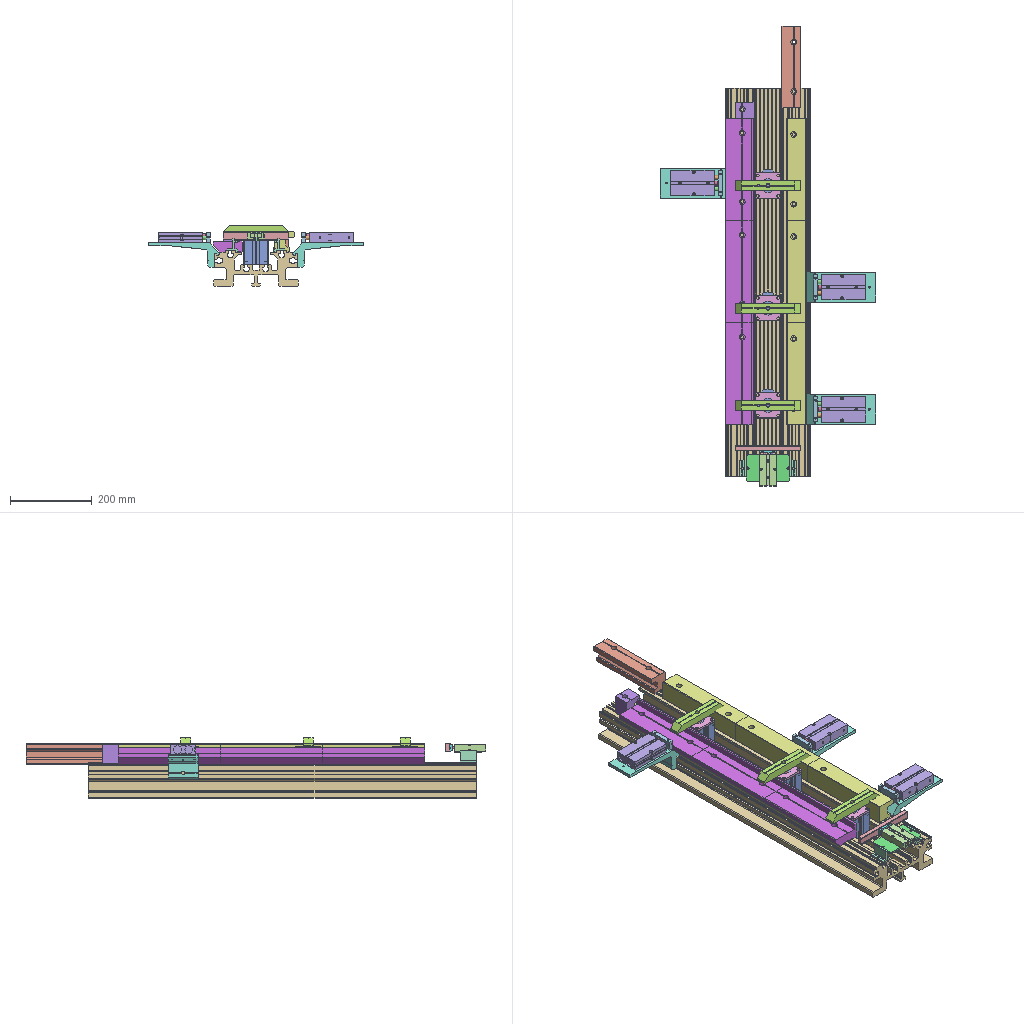Assembly | NX | 14 different items | 29 placed | box 528 x 1126 x 149 mm
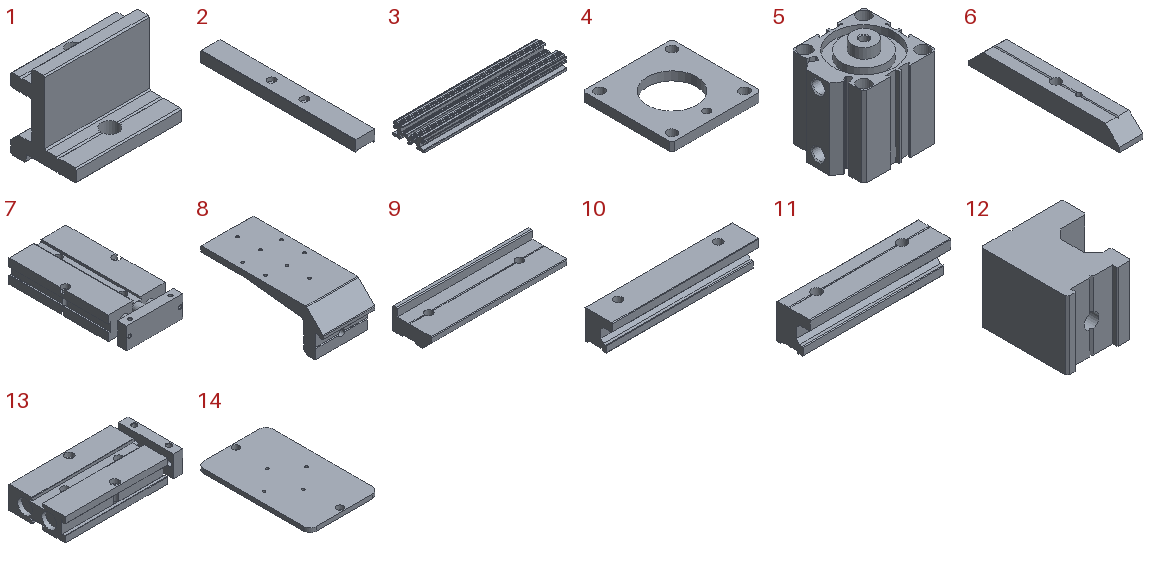Parts list (item | quantity | size | volume | features):
1 | x2 | 40 x 25.175 x 32.3 mm | 11675 mm3 | features DATUM_CSYS 3, EXTRUDE 3, SKETCH 2
2 | x1 | 20.2 x 160 x 11.5 mm | 32690 mm3 | features EXTRUDE 3, DATUM_CSYS 1
3 | x1 | 950 x 207.383 x 87 mm | 7328516 mm3 | features DATUM_CSYS 1, EXTRUDE 1
4 | x3 | 62 x 62 x 6 mm | 16618 mm3 | features EXTRUDE 2, DATUM_CSYS 1
5 | x3 | 70 x 62 x 76.6 mm | 239161 mm3 | features EXTRUDE 7, DATUM_CSYS 5, SKETCH 4, SIMPLE HOLE 3, SYMBOLIC_THREAD 3, HOLE PACKAGE 2
6 | x3 | 25 x 160 x 19.5 mm | 70356 mm3 | features EXTRUDE 3, DATUM_CSYS 1
7 | x3 | 62 x 128 x 25 mm | 171268 mm3 | features EXTRUDE 10, DATUM_CSYS 9, SKETCH 9, SIMPLE HOLE 8, SYMBOLIC_THREAD 8, HOLE PACKAGE 4, BLEND 1
8 | x3 | 73 x 173.8 x 59.75 mm | 188339 mm3 | features SIMPLE HOLE 8, SYMBOLIC_THREAD 8, DATUM_CSYS 3, EXTRUDE 2, SKETCH 2, HOLE PACKAGE 1
9 | x3 | 250 x 72 x 41.5 mm | 446626 mm3 | features EXTRUDE 3, DATUM_CSYS 2, SKETCH 1
10 | x3 | 250 x 47 x 50 mm | 417029 mm3 | features EXTRUDE 3, DATUM_CSYS 2, SKETCH 1
11 | x1 | 200 x 47 x 50 mm | 331921 mm3 | features EXTRUDE 3, DATUM_CSYS 2, SKETCH 1
12 | x1 | 47 x 50 x 39.5 mm | 63249 mm3 | features EXTRUDE 3, DATUM_CSYS 2, SKETCH 1
13 | x1 | 88.3 x 42 x 17 mm | 51096 mm3 | features DATUM_CSYS 9, SKETCH 8, SIMPLE HOLE 6, SYMBOLIC_THREAD 4, EXTRUDE 3, HOLE PACKAGE 3, BREP 1
14 | x1 | 65 x 106.527 x 4 mm | 27252 mm3 | features MOVE_FACE 2, DATUM_CSYS 1, EXTRUDE 1
Mates (type | each side: item.copy, entity, surface, feature):
Fix | 3.1 component
Bond | 1.1 component | 14.1 component | 13.1 component | 2.1 component | 1.1 component
Center22 | 1.1 face plane Extrude(1) | 1.1 face plane Extrude(1) | 3.1 face plane Extrude(1) | 3.1 face plane Extrude(1)
Touch | 1.1 face plane Extrude(1) | 3.1 face plane Extrude(1) | 2 times
Touch | 10.1 face plane Extrude(1) | 3.1 face plane Extrude(1)
Center22 | 10.1 face plane Extrude(1) | 10.1 face plane Extrude(1) | 3.1 face plane Extrude(1) | 3.1 face plane Extrude(1)
Distance | 10.1 face plane Extrude(1) | 2.1 face plane Extrude(1)
Touch | 8.1 face plane Extrude(1) | 3.1 face plane Extrude(1) | 4 times
Bond | 7.1 component | 8.1 component | 2 times
Center22 | 9.1 face plane Extrude(1) | 9.1 face plane Extrude(1) | 3.1 face plane Extrude(1) | 3.1 face plane Extrude(1)
Touch | 9.1 face plane Extrude(1) | 3.1 face plane Extrude(1)
Distance | 9.1 face plane Extrude(1) | 2.1 face plane Extrude(1)
Touch | 5.1 face plane Extrude(2) | 3.1 face plane Extrude(1)
Center22 | 5.1 face plane Extrude(2) | 5.1 face plane Extrude(2) | 3.1 face plane Extrude(1) | 3.1 face plane Extrude(1)
Bond | 6.1 component | 4.1 component | 5.1 component | 3 times
Touch | 12.1 face plane Extrude(1) | 3.1 face plane Extrude(1)
Center22 | 12.1 face plane Extrude(1) | 12.1 face plane Extrude(1) | 3.1 face plane Extrude(1) | 3.1 face plane Extrude(1)
Touch | 12.1 face plane Extrude(1) | 9.1 face plane Extrude(1)
Touch | 11.1 face plane Extrude(1) | 3.1 face plane Extrude(1)
Center22 | 11.1 face plane Extrude(1) | 11.1 face plane Extrude(1) | 3.1 face plane Extrude(1) | 3.1 face plane Extrude(1)